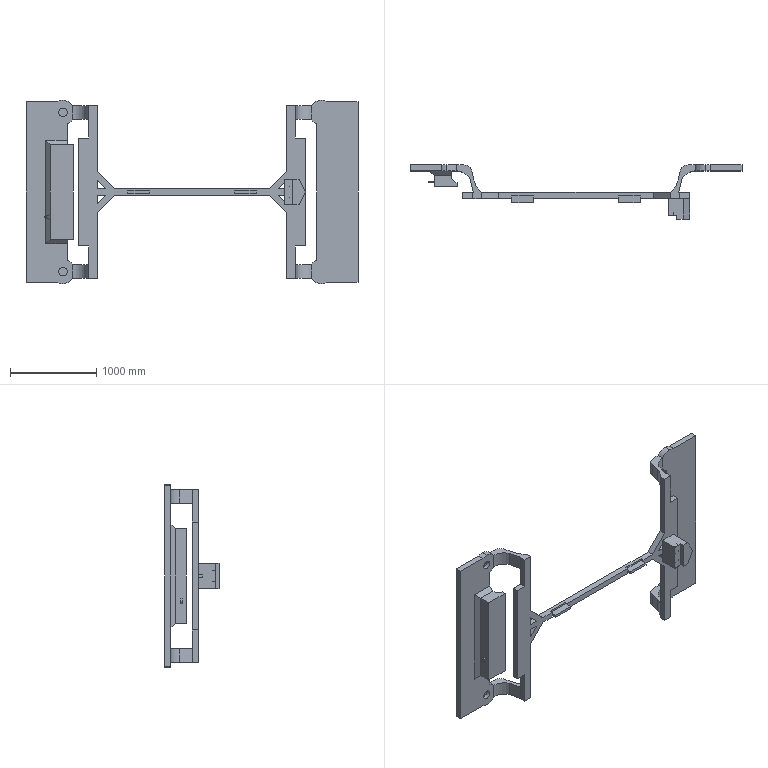Part | STEP file | Chassis | 2 solids | 170 faces | box 3860 x 630 x 2130 mm | volume 286011654 mm3 | plane 121 | cylinder 49 | commonest cylinder face diameters 4.2 x16 280 x12 100 x4 200 x4 360 x4 500 x4